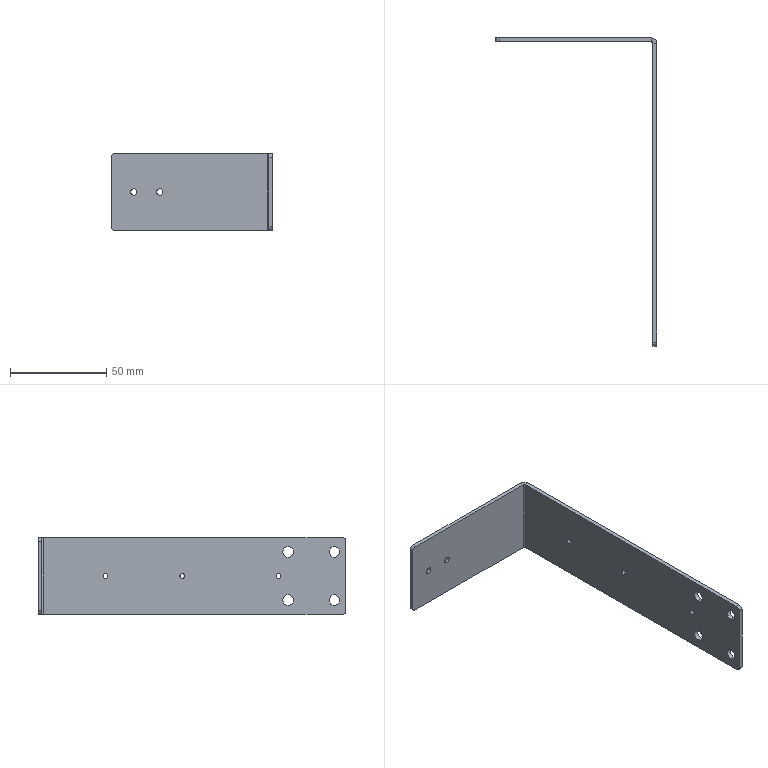Part | STEP file | 0-19-20 Drag chain bracket | 1 solid | 36 faces | box 84 x 160 x 40 mm | volume 19040 mm3 | cylinder 24 | plane 12 | commonest cylinder face diameters 5.5 x8 2.5 x6 3.3 x4 4 x4 1.473 x1 5.473 x1